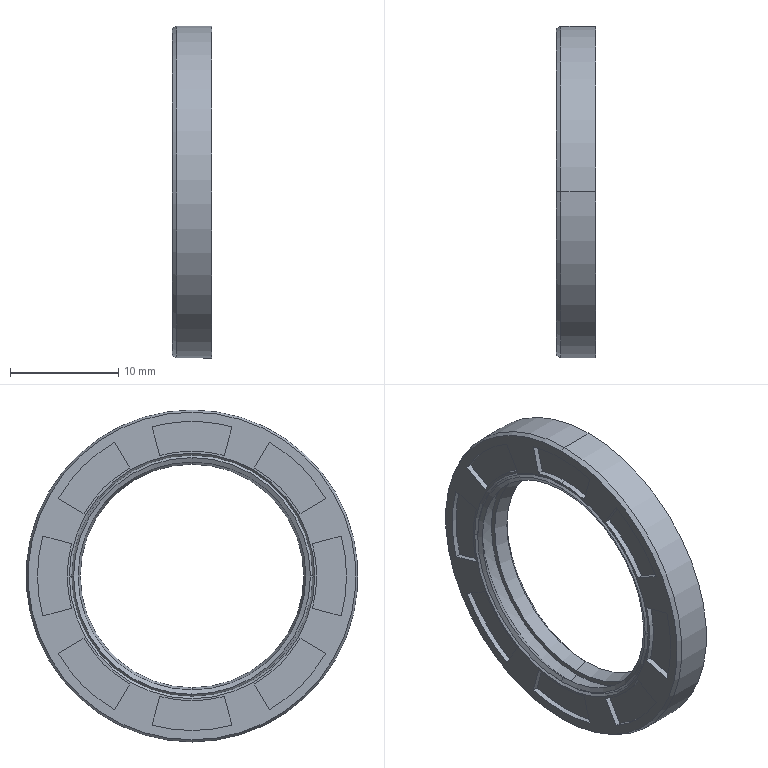Part | STEP file | _X2_6cb95c01_X0_20X30X4_5.STEP.STEP | 1 solid | 68 faces | box 3.6 x 30.624 x 30.624 mm | volume 1217 mm3 | plane 32 | cylinder 20 | cone 16 | commonest cylinder face diameters 23 x9 28.5 x9 30.624 x2